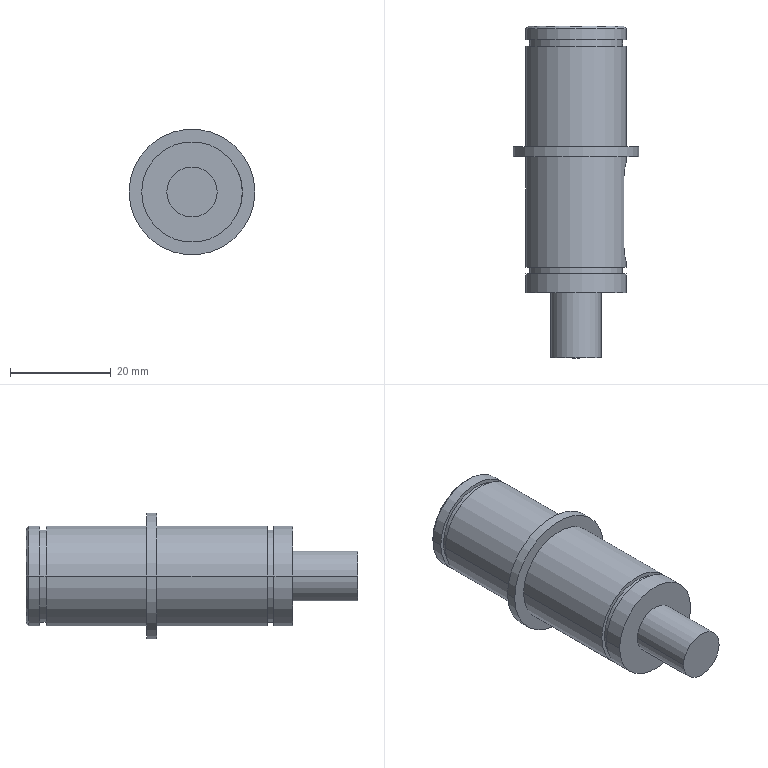Part | NX | features BREP 1 | 1 solid | 33 faces | box 25 x 66 x 25 mm | volume 17523 mm3 | cylinder 19 | plane 12 | cone 2 | commonest cylinder face diameters 20 x8 18.5 x4 6 x3 10 x2 25 x2
STEP:
#1=CARTESIAN_POINT('',(-9.5,66.,0.));
#2=VERTEX_POINT('',#1);
#3=CARTESIAN_POINT('',(9.5,66.,0.));
#4=VERTEX_POINT('',#3);
#5=CARTESIAN_POINT('',(0.,66.,0.));
#6=DIRECTION('',(0.,1.,0.));
#7=DIRECTION('',(-1.,0.,0.));
#8=AXIS2_PLACEMENT_3D('',#5,#6,#7);
#9=CIRCLE('',#8,9.5);
#10=EDGE_CURVE('',#2,#4,#9,.T.);
#11=ORIENTED_EDGE('',*,*,#10,.F.);
#12=CARTESIAN_POINT('',(-10.,65.5,0.));
#13=VERTEX_POINT('',#12);
#14=CARTESIAN_POINT('',(-10.,65.5,0.));
#15=DIRECTION('',(-0.7071,-0.7071,0.));
#16=VECTOR('',#15,1000.);
#17=LINE('',#14,#16);
#18=EDGE_CURVE('',#2,#13,#17,.T.);
#19=ORIENTED_EDGE('',*,*,#18,.T.);
#20=CARTESIAN_POINT('',(10.,65.5,0.));
#21=VERTEX_POINT('',#20);
#22=CARTESIAN_POINT('',(0.,65.5,0.));
#23=DIRECTION('',(0.,-1.,0.));
#24=DIRECTION('',(-1.,0.,0.));
#25=AXIS2_PLACEMENT_3D('',#22,#23,#24);
#26=CIRCLE('',#25,10.);
#27=EDGE_CURVE('',#21,#13,#26,.T.);
#28=ORIENTED_EDGE('',*,*,#27,.F.);
#29=CARTESIAN_POINT('',(10.,65.5,0.));
#30=DIRECTION('',(0.7071,-0.7071,0.));
#31=VECTOR('',#30,1000.);
#32=LINE('',#29,#31);
#33=EDGE_CURVE('',#4,#21,#32,.T.);
#34=ORIENTED_EDGE('',*,*,#33,.F.);
#35=EDGE_LOOP('',(#11,#19,#28,#34));
#36=FACE_BOUND('',#35,.T.);
#37=CARTESIAN_POINT('',(0.,65.5,0.));
#38=DIRECTION('',(0.,-1.,0.));
#39=DIRECTION('',(-1.,0.,0.));
#40=AXIS2_PLACEMENT_3D('',#37,#38,#39);
#41=CONICAL_SURFACE('',#40,10.,0.7854);
#42=ADVANCED_FACE('',(#36),#41,.T.);
#43=ORIENTED_EDGE('',*,*,#27,.T.);
#44=CARTESIAN_POINT('',(-10.,63.3,0.));
#45=VERTEX_POINT('',#44);
#46=CARTESIAN_POINT('',(-10.,0.,0.));
#47=DIRECTION('',(0.,-1.,0.));
#48=VECTOR('',#47,1000.);
#49=LINE('',#46,#48);
#50=EDGE_CURVE('',#13,#45,#49,.T.);
#51=ORIENTED_EDGE('',*,*,#50,.T.);
#52=CARTESIAN_POINT('',(10.,63.3,0.));
#53=VERTEX_POINT('',#52);
#54=CARTESIAN_POINT('',(0.,63.3,0.));
#55=DIRECTION('',(0.,-1.,0.));
#56=DIRECTION('',(1.,0.,0.));
#57=AXIS2_PLACEMENT_3D('',#54,#55,#56);
#58=CIRCLE('',#57,10.);
#59=EDGE_CURVE('',#53,#45,#58,.T.);
#60=ORIENTED_EDGE('',*,*,#59,.F.);
#61=CARTESIAN_POINT('',(10.,0.,0.));
#62=DIRECTION('',(0.,-1.,0.));
#63=VECTOR('',#62,1000.);
#64=LINE('',#61,#63);
#65=EDGE_CURVE('',#21,#53,#64,.T.);
#66=ORIENTED_EDGE('',*,*,#65,.F.);
#67=EDGE_LOOP('',(#43,#51,#60,#66));
#68=FACE_BOUND('',#67,.T.);
#69=CARTESIAN_POINT('',(0.,0.,0.));
#70=DIRECTION('',(0.,-1.,0.));
#71=DIRECTION('',(-1.,0.,0.));
#72=AXIS2_PLACEMENT_3D('',#69,#70,#71);
#73=CYLINDRICAL_SURFACE('',#72,10.);
#74=ADVANCED_FACE('',(#68),#73,.T.);
#75=CARTESIAN_POINT('',(9.25,62.,0.));
#76=VERTEX_POINT('',#75);
#77=CARTESIAN_POINT('',(-9.25,62.,0.));
#78=VERTEX_POINT('',#77);
#79=CARTESIAN_POINT('',(0.,62.,0.));
#80=DIRECTION('',(0.,-1.,0.));
#81=DIRECTION('',(1.,0.,0.));
#82=AXIS2_PLACEMENT_3D('',#79,#80,#81);
#83=CIRCLE('',#82,9.25);
#84=EDGE_CURVE('',#76,#78,#83,.T.);
#85=ORIENTED_EDGE('',*,*,#84,.F.);
#86=CARTESIAN_POINT('',(9.25,63.3,0.));
#87=VERTEX_POINT('',#86);
#88=CARTESIAN_POINT('',(9.25,62.,0.));
#89=DIRECTION('',(0.,1.,0.));
#90=VECTOR('',#89,1000.);
#91=LINE('',#88,#90);
#92=EDGE_CURVE('',#87,#76,#91,.F.);
#93=ORIENTED_EDGE('',*,*,#92,.F.);
#94=CARTESIAN_POINT('',(-9.25,63.3,0.));
#95=VERTEX_POINT('',#94);
#96=CARTESIAN_POINT('',(0.,63.3,0.));
#97=DIRECTION('',(0.,-1.,0.));
#98=DIRECTION('',(1.,0.,0.));
#99=AXIS2_PLACEMENT_3D('',#96,#97,#98);
#100=CIRCLE('',#99,9.25);
#101=EDGE_CURVE('',#87,#95,#100,.T.);
#102=ORIENTED_EDGE('',*,*,#101,.T.);
#103=CARTESIAN_POINT('',(-9.25,62.,0.));
#104=DIRECTION('',(0.,1.,0.));
#105=VECTOR('',#104,1000.);
#106=LINE('',#103,#105);
#107=EDGE_CURVE('',#95,#78,#106,.F.);
#108=ORIENTED_EDGE('',*,*,#107,.T.);
#109=EDGE_LOOP('',(#85,#93,#102,#108));
#110=FACE_BOUND('',#109,.T.);
#111=CARTESIAN_POINT('',(0.,62.,0.));
#112=DIRECTION('',(0.,1.,0.));
#113=DIRECTION('',(1.,0.,0.));
#114=AXIS2_PLACEMENT_3D('',#111,#112,#113);
#115=CYLINDRICAL_SURFACE('',#114,9.25);
#116=ADVANCED_FACE('',(#110),#115,.T.);
#117=CARTESIAN_POINT('',(10.,16.7,0.));
#118=VERTEX_POINT('',#117);
#119=CARTESIAN_POINT('',(-10.,16.7,0.));
#120=VERTEX_POINT('',#119);
#121=CARTESIAN_POINT('',(0.,16.7,0.));
#122=DIRECTION('',(0.,-1.,0.));
#123=DIRECTION('',(1.,0.,0.));
#124=AXIS2_PLACEMENT_3D('',#121,#122,#123);
#125=CIRCLE('',#124,10.);
#126=EDGE_CURVE('',#118,#120,#125,.T.);
#127=ORIENTED_EDGE('',*,*,#126,.T.);
#128=CARTESIAN_POINT('',(-10.,13.,0.));
#129=VERTEX_POINT('',#128);
#130=CARTESIAN_POINT('',(-10.,0.,0.));
#131=DIRECTION('',(0.,-1.,0.));
#132=VECTOR('',#131,1000.);
#133=LINE('',#130,#132);
#134=EDGE_CURVE('',#120,#129,#133,.T.);
#135=ORIENTED_EDGE('',*,*,#134,.T.);
#136=CARTESIAN_POINT('',(10.,13.,0.));
#137=VERTEX_POINT('',#136);
#138=CARTESIAN_POINT('',(0.,13.,0.));
#139=DIRECTION('',(0.,-1.,0.));
#140=DIRECTION('',(1.,0.,0.));
#141=AXIS2_PLACEMENT_3D('',#138,#139,#140);
#142=CIRCLE('',#141,10.);
#143=EDGE_CURVE('',#137,#129,#142,.T.);
#144=ORIENTED_EDGE('',*,*,#143,.F.);
#145=CARTESIAN_POINT('',(10.,0.,0.));
#146=DIRECTION('',(0.,-1.,0.));
#147=VECTOR('',#146,1000.);
#148=LINE('',#145,#147);
#149=EDGE_CURVE('',#118,#137,#148,.T.);
#150=ORIENTED_EDGE('',*,*,#149,.F.);
#151=EDGE_LOOP('',(#127,#135,#144,#150));
#152=FACE_BOUND('',#151,.T.);
#153=CARTESIAN_POINT('',(0.,0.,0.));
#154=DIRECTION('',(0.,-1.,0.));
#155=DIRECTION('',(-1.,0.,0.));
#156=AXIS2_PLACEMENT_3D('',#153,#154,#155);
#157=CYLINDRICAL_SURFACE('',#156,10.);
#158=ADVANCED_FACE('',(#152),#157,.T.);
#159=CARTESIAN_POINT('',(5.,13.,0.));
#160=VERTEX_POINT('',#159);
#161=CARTESIAN_POINT('',(-5.,13.,0.));
#162=VERTEX_POINT('',#161);
#163=CARTESIAN_POINT('',(0.,13.,0.));
#164=DIRECTION('',(0.,-1.,0.));
#165=DIRECTION('',(1.,0.,0.));
#166=AXIS2_PLACEMENT_3D('',#163,#164,#165);
#167=CIRCLE('',#166,5.);
#168=EDGE_CURVE('',#160,#162,#167,.T.);
#169=ORIENTED_EDGE('',*,*,#168,.T.);
#170=CARTESIAN_POINT('',(-5.,0.,0.));
#171=VERTEX_POINT('',#170);
#172=CARTESIAN_POINT('',(-5.,0.,0.));
#173=DIRECTION('',(0.,-1.,0.));
#174=VECTOR('',#173,1000.);
#175=LINE('',#172,#174);
#176=EDGE_CURVE('',#162,#171,#175,.T.);
#177=ORIENTED_EDGE('',*,*,#176,.T.);
#178=CARTESIAN_POINT('',(5.,0.,0.));
#179=VERTEX_POINT('',#178);
#180=CARTESIAN_POINT('',(0.,0.,0.));
#181=DIRECTION('',(0.,-1.,0.));
#182=DIRECTION('',(1.,0.,0.));
#183=AXIS2_PLACEMENT_3D('',#180,#181,#182);
#184=CIRCLE('',#183,5.);
#185=EDGE_CURVE('',#179,#171,#184,.T.);
#186=ORIENTED_EDGE('',*,*,#185,.F.);
#187=CARTESIAN_POINT('',(5.,0.,0.));
#188=DIRECTION('',(0.,-1.,0.));
#189=VECTOR('',#188,1000.);
#190=LINE('',#187,#189);
#191=EDGE_CURVE('',#160,#179,#190,.T.);
#192=ORIENTED_EDGE('',*,*,#191,.F.);
#193=EDGE_LOOP('',(#169,#177,#186,#192));
#194=FACE_BOUND('',#193,.T.);
#195=CARTESIAN_POINT('',(0.,0.,0.));
#196=DIRECTION('',(0.,-1.,0.));
#197=DIRECTION('',(-1.,0.,0.));
#198=AXIS2_PLACEMENT_3D('',#195,#196,#197);
#199=CYLINDRICAL_SURFACE('',#198,5.);
#200=ADVANCED_FACE('',(#194),#199,.T.);
#201=CARTESIAN_POINT('',(9.25,16.7,0.));
#202=VERTEX_POINT('',#201);
#203=CARTESIAN_POINT('',(-9.25,16.7,0.));
#204=VERTEX_POINT('',#203);
#205=CARTESIAN_POINT('',(0.,16.7,0.));
#206=DIRECTION('',(0.,-1.,0.));
#207=DIRECTION('',(1.,0.,0.));
#208=AXIS2_PLACEMENT_3D('',#205,#206,#207);
#209=CIRCLE('',#208,9.25);
#210=EDGE_CURVE('',#202,#204,#209,.T.);
#211=ORIENTED_EDGE('',*,*,#210,.F.);
#212=CARTESIAN_POINT('',(9.25,18.,0.));
#213=VERTEX_POINT('',#212);
#214=CARTESIAN_POINT('',(9.25,16.7,0.));
#215=DIRECTION('',(0.,1.,0.));
#216=VECTOR('',#215,1000.);
#217=LINE('',#214,#216);
#218=EDGE_CURVE('',#213,#202,#217,.F.);
#219=ORIENTED_EDGE('',*,*,#218,.F.);
#220=CARTESIAN_POINT('',(-9.25,18.,0.));
#221=VERTEX_POINT('',#220);
#222=CARTESIAN_POINT('',(0.,18.,0.));
#223=DIRECTION('',(0.,-1.,0.));
#224=DIRECTION('',(1.,0.,0.));
#225=AXIS2_PLACEMENT_3D('',#222,#223,#224);
#226=CIRCLE('',#225,9.25);
#227=EDGE_CURVE('',#213,#221,#226,.T.);
#228=ORIENTED_EDGE('',*,*,#227,.T.);
#229=CARTESIAN_POINT('',(-9.25,16.7,0.));
#230=DIRECTION('',(0.,1.,0.));
#231=VECTOR('',#230,1000.);
#232=LINE('',#229,#231);
#233=EDGE_CURVE('',#221,#204,#232,.F.);
#234=ORIENTED_EDGE('',*,*,#233,.T.);
#235=EDGE_LOOP('',(#211,#219,#228,#234));
#236=FACE_BOUND('',#235,.T.);
#237=CARTESIAN_POINT('',(0.,16.7,0.));
#238=DIRECTION('',(0.,1.,0.));
#239=DIRECTION('',(1.,0.,0.));
#240=AXIS2_PLACEMENT_3D('',#237,#238,#239);
#241=CYLINDRICAL_SURFACE('',#240,9.25);
#242=ADVANCED_FACE('',(#236),#241,.T.);
#243=CARTESIAN_POINT('',(6.5,39.,0.));
#244=VERTEX_POINT('',#243);
#245=CARTESIAN_POINT('',(6.5,36.,3.));
#246=VERTEX_POINT('',#245);
#247=CARTESIAN_POINT('',(6.5,36.,0.));
#248=DIRECTION('',(1.,0.,0.));
#249=DIRECTION('',(0.,1.,0.));
#250=AXIS2_PLACEMENT_3D('',#247,#248,#249);
#251=CIRCLE('',#250,3.);
#252=EDGE_CURVE('',#244,#246,#251,.T.);
#253=ORIENTED_EDGE('',*,*,#252,.F.);
#254=CARTESIAN_POINT('',(10.,39.,0.));
#255=VERTEX_POINT('',#254);
#256=CARTESIAN_POINT('',(6.5,39.,0.));
#257=DIRECTION('',(1.,0.,0.));
#258=VECTOR('',#257,1000.);
#259=LINE('',#256,#258);
#260=EDGE_CURVE('',#244,#255,#259,.T.);
#261=ORIENTED_EDGE('',*,*,#260,.T.);
#262=CARTESIAN_POINT('',(9.539,36.,3.));
#263=VERTEX_POINT('',#262);
#264=CARTESIAN_POINT('',(10.,39.,0.));
#265=CARTESIAN_POINT('',(10.,39.,0.7973));
#266=CARTESIAN_POINT('',(9.775,38.345,2.343));
#267=CARTESIAN_POINT('',(9.539,36.797,3.));
#268=CARTESIAN_POINT('',(9.539,36.,3.));
#269=B_SPLINE_CURVE_WITH_KNOTS('',3,(#264,#265,#266,#267,#268),.UNSPECIFIED.,.F.,.F.,(4,1,4),(0.,0.002357,0.004714),.UNSPECIFIED.);
#270=EDGE_CURVE('',#255,#263,#269,.T.);
#271=ORIENTED_EDGE('',*,*,#270,.T.);
#272=CARTESIAN_POINT('',(6.5,36.,3.));
#273=DIRECTION('',(1.,0.,0.));
#274=VECTOR('',#273,1000.);
#275=LINE('',#272,#274);
#276=EDGE_CURVE('',#246,#263,#275,.T.);
#277=ORIENTED_EDGE('',*,*,#276,.F.);
#278=EDGE_LOOP('',(#253,#261,#271,#277));
#279=FACE_BOUND('',#278,.T.);
#280=CARTESIAN_POINT('',(6.5,36.,0.));
#281=DIRECTION('',(1.,0.,0.));
#282=DIRECTION('',(0.,-1.,0.));
#283=AXIS2_PLACEMENT_3D('',#280,#281,#282);
#284=CYLINDRICAL_SURFACE('',#283,3.);
#285=ADVANCED_FACE('',(#279),#284,.F.);
#286=CARTESIAN_POINT('',(12.5,42.,0.));
#287=VERTEX_POINT('',#286);
#288=CARTESIAN_POINT('',(-12.5,42.,0.));
#289=VERTEX_POINT('',#288);
#290=CARTESIAN_POINT('',(0.,42.,0.));
#291=DIRECTION('',(0.,-1.,0.));
#292=DIRECTION('',(1.,0.,0.));
#293=AXIS2_PLACEMENT_3D('',#290,#291,#292);
#294=CIRCLE('',#293,12.5);
#295=EDGE_CURVE('',#287,#289,#294,.T.);
#296=ORIENTED_EDGE('',*,*,#295,.T.);
#297=CARTESIAN_POINT('',(-12.5,40.,0.));
#298=VERTEX_POINT('',#297);
#299=CARTESIAN_POINT('',(-12.5,0.,0.));
#300=DIRECTION('',(0.,-1.,0.));
#301=VECTOR('',#300,1000.);
#302=LINE('',#299,#301);
#303=EDGE_CURVE('',#289,#298,#302,.T.);
#304=ORIENTED_EDGE('',*,*,#303,.T.);
#305=CARTESIAN_POINT('',(12.5,40.,0.));
#306=VERTEX_POINT('',#305);
#307=CARTESIAN_POINT('',(0.,40.,0.));
#308=DIRECTION('',(0.,-1.,0.));
#309=DIRECTION('',(1.,0.,0.));
#310=AXIS2_PLACEMENT_3D('',#307,#308,#309);
#311=CIRCLE('',#310,12.5);
#312=EDGE_CURVE('',#306,#298,#311,.T.);
#313=ORIENTED_EDGE('',*,*,#312,.F.);
#314=CARTESIAN_POINT('',(12.5,0.,0.));
#315=DIRECTION('',(0.,-1.,0.));
#316=VECTOR('',#315,1000.);
#317=LINE('',#314,#316);
#318=EDGE_CURVE('',#287,#306,#317,.T.);
#319=ORIENTED_EDGE('',*,*,#318,.F.);
#320=EDGE_LOOP('',(#296,#304,#313,#319));
#321=FACE_BOUND('',#320,.T.);
#322=CARTESIAN_POINT('',(0.,0.,0.));
#323=DIRECTION('',(0.,-1.,0.));
#324=DIRECTION('',(-1.,0.,0.));
#325=AXIS2_PLACEMENT_3D('',#322,#323,#324);
#326=CYLINDRICAL_SURFACE('',#325,12.5);
#327=ADVANCED_FACE('',(#321),#326,.T.);
#328=CARTESIAN_POINT('',(10.,62.,0.));
#329=VERTEX_POINT('',#328);
#330=CARTESIAN_POINT('',(-10.,62.,0.));
#331=VERTEX_POINT('',#330);
#332=CARTESIAN_POINT('',(0.,62.,0.));
#333=DIRECTION('',(0.,-1.,0.));
#334=DIRECTION('',(1.,0.,0.));
#335=AXIS2_PLACEMENT_3D('',#332,#333,#334);
#336=CIRCLE('',#335,10.);
#337=EDGE_CURVE('',#329,#331,#336,.T.);
#338=ORIENTED_EDGE('',*,*,#337,.T.);
#339=CARTESIAN_POINT('',(-10.,42.,0.));
#340=VERTEX_POINT('',#339);
#341=CARTESIAN_POINT('',(-10.,0.,0.));
#342=DIRECTION('',(0.,-1.,0.));
#343=VECTOR('',#342,1000.);
#344=LINE('',#341,#343);
#345=EDGE_CURVE('',#331,#340,#344,.T.);
#346=ORIENTED_EDGE('',*,*,#345,.T.);
#347=CARTESIAN_POINT('',(10.,42.,0.));
#348=VERTEX_POINT('',#347);
#349=CARTESIAN_POINT('',(0.,42.,0.));
#350=DIRECTION('',(0.,-1.,0.));
#351=DIRECTION('',(1.,0.,0.));
#352=AXIS2_PLACEMENT_3D('',#349,#350,#351);
#353=CIRCLE('',#352,10.);
#354=EDGE_CURVE('',#348,#340,#353,.T.);
#355=ORIENTED_EDGE('',*,*,#354,.F.);
#356=CARTESIAN_POINT('',(10.,0.,0.));
#357=DIRECTION('',(0.,-1.,0.));
#358=VECTOR('',#357,1000.);
#359=LINE('',#356,#358);
#360=EDGE_CURVE('',#329,#348,#359,.T.);
#361=ORIENTED_EDGE('',*,*,#360,.F.);
#362=EDGE_LOOP('',(#338,#346,#355,#361));
#363=FACE_BOUND('',#362,.T.);
#364=CARTESIAN_POINT('',(0.,0.,0.));
#365=DIRECTION('',(0.,-1.,0.));
#366=DIRECTION('',(-1.,0.,0.));
#367=AXIS2_PLACEMENT_3D('',#364,#365,#366);
#368=CYLINDRICAL_SURFACE('',#367,10.);
#369=ADVANCED_FACE('',(#363),#368,.T.);
#370=CARTESIAN_POINT('',(10.,40.,0.));
#371=VERTEX_POINT('',#370);
#372=CARTESIAN_POINT('',(-10.,40.,0.));
#373=VERTEX_POINT('',#372);
#374=CARTESIAN_POINT('',(0.,40.,0.));
#375=DIRECTION('',(0.,-1.,0.));
#376=DIRECTION('',(1.,0.,0.));
#377=AXIS2_PLACEMENT_3D('',#374,#375,#376);
#378=CIRCLE('',#377,10.);
#379=EDGE_CURVE('',#371,#373,#378,.T.);
#380=ORIENTED_EDGE('',*,*,#379,.T.);
#381=CARTESIAN_POINT('',(-10.,18.,0.));
#382=VERTEX_POINT('',#381);
#383=CARTESIAN_POINT('',(-10.,0.,0.));
#384=DIRECTION('',(0.,-1.,0.));
#385=VECTOR('',#384,1000.);
#386=LINE('',#383,#385);
#387=EDGE_CURVE('',#373,#382,#386,.T.);
#388=ORIENTED_EDGE('',*,*,#387,.T.);
#389=CARTESIAN_POINT('',(10.,18.,0.));
#390=VERTEX_POINT('',#389);
#391=CARTESIAN_POINT('',(0.,18.,0.));
#392=DIRECTION('',(0.,-1.,0.));
#393=DIRECTION('',(1.,0.,0.));
#394=AXIS2_PLACEMENT_3D('',#391,#392,#393);
#395=CIRCLE('',#394,10.);
#396=EDGE_CURVE('',#390,#382,#395,.T.);
#397=ORIENTED_EDGE('',*,*,#396,.F.);
#398=CARTESIAN_POINT('',(10.,19.,0.));
#399=VERTEX_POINT('',#398);
#400=CARTESIAN_POINT('',(10.,0.,0.));
#401=DIRECTION('',(0.,-1.,0.));
#402=VECTOR('',#401,1000.);
#403=LINE('',#400,#402);
#404=EDGE_CURVE('',#399,#390,#403,.T.);
#405=ORIENTED_EDGE('',*,*,#404,.F.);
#406=CARTESIAN_POINT('',(9.539,22.,3.));
#407=VERTEX_POINT('',#406);
#408=CARTESIAN_POINT('',(9.539,22.,3.));
#409=CARTESIAN_POINT('',(9.539,21.203,3.));
#410=CARTESIAN_POINT('',(9.775,19.657,2.345));
#411=CARTESIAN_POINT('',(10.,19.,0.7973));
#412=CARTESIAN_POINT('',(10.,19.,0.));
#413=B_SPLINE_CURVE_WITH_KNOTS('',3,(#408,#409,#410,#411,#412),.UNSPECIFIED.,.F.,.F.,(4,1,4),(0.,0.002357,0.004714),.UNSPECIFIED.);
#414=EDGE_CURVE('',#407,#399,#413,.T.);
#415=ORIENTED_EDGE('',*,*,#414,.F.);
#416=CARTESIAN_POINT('',(9.539,0.,3.));
#417=DIRECTION('',(0.,-1.,0.));
#418=VECTOR('',#417,1000.);
#419=LINE('',#416,#418);
#420=EDGE_CURVE('',#263,#407,#419,.T.);
#421=ORIENTED_EDGE('',*,*,#420,.F.);
#422=ORIENTED_EDGE('',*,*,#270,.F.);
#423=CARTESIAN_POINT('',(10.,0.,0.));
#424=DIRECTION('',(0.,-1.,0.));
#425=VECTOR('',#424,1000.);
#426=LINE('',#423,#425);
#427=EDGE_CURVE('',#371,#255,#426,.T.);
#428=ORIENTED_EDGE('',*,*,#427,.F.);
#429=EDGE_LOOP('',(#380,#388,#397,#405,#415,#421,#422,#428));
#430=FACE_BOUND('',#429,.T.);
#431=CARTESIAN_POINT('',(0.,0.,0.));
#432=DIRECTION('',(0.,-1.,0.));
#433=DIRECTION('',(-1.,0.,0.));
#434=AXIS2_PLACEMENT_3D('',#431,#432,#433);
#435=CYLINDRICAL_SURFACE('',#434,10.);
#436=ADVANCED_FACE('',(#430),#435,.T.);
#437=ORIENTED_EDGE('',*,*,#387,.F.);
#438=CARTESIAN_POINT('',(0.,40.,0.));
#439=DIRECTION('',(0.,-1.,0.));
#440=DIRECTION('',(1.,0.,0.));
#441=AXIS2_PLACEMENT_3D('',#438,#439,#440);
#442=CIRCLE('',#441,10.);
#443=EDGE_CURVE('',#373,#371,#442,.T.);
#444=ORIENTED_EDGE('',*,*,#443,.T.);
#445=ORIENTED_EDGE('',*,*,#427,.T.);
#446=CARTESIAN_POINT('',(9.539,36.,-3.));
#447=VERTEX_POINT('',#446);
#448=CARTESIAN_POINT('',(9.539,36.,-3.));
#449=CARTESIAN_POINT('',(9.539,36.797,-3.));
#450=CARTESIAN_POINT('',(9.775,38.343,-2.345));
#451=CARTESIAN_POINT('',(10.,39.,-0.7973));
#452=CARTESIAN_POINT('',(10.,39.,0.));
#453=B_SPLINE_CURVE_WITH_KNOTS('',3,(#448,#449,#450,#451,#452),.UNSPECIFIED.,.F.,.F.,(4,1,4),(0.,0.002357,0.004714),.UNSPECIFIED.);
#454=EDGE_CURVE('',#447,#255,#453,.T.);
#455=ORIENTED_EDGE('',*,*,#454,.F.);
#456=CARTESIAN_POINT('',(9.539,22.,-3.));
#457=VERTEX_POINT('',#456);
#458=CARTESIAN_POINT('',(9.539,0.,-3.));
#459=DIRECTION('',(0.,1.,0.));
#460=VECTOR('',#459,1000.);
#461=LINE('',#458,#460);
#462=EDGE_CURVE('',#457,#447,#461,.T.);
#463=ORIENTED_EDGE('',*,*,#462,.F.);
#464=CARTESIAN_POINT('',(10.,19.,0.));
#465=CARTESIAN_POINT('',(10.,19.,-0.7973));
#466=CARTESIAN_POINT('',(9.775,19.655,-2.343));
#467=CARTESIAN_POINT('',(9.539,21.203,-3.));
#468=CARTESIAN_POINT('',(9.539,22.,-3.));
#469=B_SPLINE_CURVE_WITH_KNOTS('',3,(#464,#465,#466,#467,#468),.UNSPECIFIED.,.F.,.F.,(4,1,4),(0.,0.002357,0.004714),.UNSPECIFIED.);
#470=EDGE_CURVE('',#399,#457,#469,.T.);
#471=ORIENTED_EDGE('',*,*,#470,.F.);
#472=ORIENTED_EDGE('',*,*,#404,.T.);
#473=CARTESIAN_POINT('',(0.,18.,0.));
#474=DIRECTION('',(0.,-1.,0.));
#475=DIRECTION('',(1.,0.,0.));
#476=AXIS2_PLACEMENT_3D('',#473,#474,#475);
#477=CIRCLE('',#476,10.);
#478=EDGE_CURVE('',#382,#390,#477,.T.);
#479=ORIENTED_EDGE('',*,*,#478,.F.);
#480=EDGE_LOOP('',(#437,#444,#445,#455,#463,#471,#472,#479));
#481=FACE_BOUND('',#480,.T.);
#482=CARTESIAN_POINT('',(0.,0.,0.));
#483=DIRECTION('',(0.,-1.,0.));
#484=DIRECTION('',(-1.,0.,0.));
#485=AXIS2_PLACEMENT_3D('',#482,#483,#484);
#486=CYLINDRICAL_SURFACE('',#485,10.);
#487=ADVANCED_FACE('',(#481),#486,.T.);
#488=ORIENTED_EDGE('',*,*,#345,.F.);
#489=CARTESIAN_POINT('',(0.,62.,0.));
#490=DIRECTION('',(0.,-1.,0.));
#491=DIRECTION('',(1.,0.,0.));
#492=AXIS2_PLACEMENT_3D('',#489,#490,#491);
#493=CIRCLE('',#492,10.);
#494=EDGE_CURVE('',#331,#329,#493,.T.);
#495=ORIENTED_EDGE('',*,*,#494,.T.);
#496=ORIENTED_EDGE('',*,*,#360,.T.);
#497=CARTESIAN_POINT('',(0.,42.,0.));
#498=DIRECTION('',(0.,-1.,0.));
#499=DIRECTION('',(1.,0.,0.));
#500=AXIS2_PLACEMENT_3D('',#497,#498,#499);
#501=CIRCLE('',#500,10.);
#502=EDGE_CURVE('',#340,#348,#501,.T.);
#503=ORIENTED_EDGE('',*,*,#502,.F.);
#504=EDGE_LOOP('',(#488,#495,#496,#503));
#505=FACE_BOUND('',#504,.T.);
#506=CARTESIAN_POINT('',(0.,0.,0.));
#507=DIRECTION('',(0.,-1.,0.));
#508=DIRECTION('',(-1.,0.,0.));
#509=AXIS2_PLACEMENT_3D('',#506,#507,#508);
#510=CYLINDRICAL_SURFACE('',#509,10.);
#511=ADVANCED_FACE('',(#505),#510,.T.);
#512=ORIENTED_EDGE('',*,*,#354,.T.);
#513=ORIENTED_EDGE('',*,*,#502,.T.);
#514=EDGE_LOOP('',(#512,#513));
#515=FACE_BOUND('',#514,.T.);
#516=ORIENTED_EDGE('',*,*,#295,.F.);
#517=CARTESIAN_POINT('',(0.,42.,0.));
#518=DIRECTION('',(0.,-1.,0.));
#519=DIRECTION('',(1.,0.,0.));
#520=AXIS2_PLACEMENT_3D('',#517,#518,#519);
#521=CIRCLE('',#520,12.5);
#522=EDGE_CURVE('',#289,#287,#521,.T.);
#523=ORIENTED_EDGE('',*,*,#522,.F.);
#524=EDGE_LOOP('',(#516,#523));
#525=FACE_BOUND('',#524,.T.);
#526=CARTESIAN_POINT('',(10.,42.,0.));
#527=DIRECTION('',(0.,1.,0.));
#528=DIRECTION('',(1.,0.,0.));
#529=AXIS2_PLACEMENT_3D('',#526,#527,#528);
#530=PLANE('',#529);
#531=ADVANCED_FACE('',(#515,#525),#530,.T.);
#532=ORIENTED_EDGE('',*,*,#303,.F.);
#533=ORIENTED_EDGE('',*,*,#522,.T.);
#534=ORIENTED_EDGE('',*,*,#318,.T.);
#535=CARTESIAN_POINT('',(0.,40.,0.));
#536=DIRECTION('',(0.,-1.,0.));
#537=DIRECTION('',(1.,0.,0.));
#538=AXIS2_PLACEMENT_3D('',#535,#536,#537);
#539=CIRCLE('',#538,12.5);
#540=EDGE_CURVE('',#298,#306,#539,.T.);
#541=ORIENTED_EDGE('',*,*,#540,.F.);
#542=EDGE_LOOP('',(#532,#533,#534,#541));
#543=FACE_BOUND('',#542,.T.);
#544=CARTESIAN_POINT('',(0.,0.,0.));
#545=DIRECTION('',(0.,-1.,0.));
#546=DIRECTION('',(-1.,0.,0.));
#547=AXIS2_PLACEMENT_3D('',#544,#545,#546);
#548=CYLINDRICAL_SURFACE('',#547,12.5);
#549=ADVANCED_FACE('',(#543),#548,.T.);
#550=ORIENTED_EDGE('',*,*,#312,.T.);
#551=ORIENTED_EDGE('',*,*,#540,.T.);
#552=EDGE_LOOP('',(#550,#551));
#553=FACE_BOUND('',#552,.T.);
#554=ORIENTED_EDGE('',*,*,#379,.F.);
#555=ORIENTED_EDGE('',*,*,#443,.F.);
#556=EDGE_LOOP('',(#554,#555));
#557=FACE_BOUND('',#556,.T.);
#558=CARTESIAN_POINT('',(12.5,40.,0.));
#559=DIRECTION('',(0.,-1.,0.));
#560=DIRECTION('',(-1.,0.,0.));
#561=AXIS2_PLACEMENT_3D('',#558,#559,#560);
#562=PLANE('',#561);
#563=ADVANCED_FACE('',(#553,#557),#562,.T.);
#564=ORIENTED_EDGE('',*,*,#260,.F.);
#565=CARTESIAN_POINT('',(6.5,36.,-3.));
#566=VERTEX_POINT('',#565);
#567=CARTESIAN_POINT('',(6.5,36.,0.));
#568=DIRECTION('',(1.,0.,0.));
#569=DIRECTION('',(0.,1.,0.));
#570=AXIS2_PLACEMENT_3D('',#567,#568,#569);
#571=CIRCLE('',#570,3.);
#572=EDGE_CURVE('',#566,#244,#571,.T.);
#573=ORIENTED_EDGE('',*,*,#572,.F.);
#574=CARTESIAN_POINT('',(6.5,36.,-3.));
#575=DIRECTION('',(1.,0.,0.));
#576=VECTOR('',#575,1000.);
#577=LINE('',#574,#576);
#578=EDGE_CURVE('',#566,#447,#577,.T.);
#579=ORIENTED_EDGE('',*,*,#578,.T.);
#580=ORIENTED_EDGE('',*,*,#454,.T.);
#581=EDGE_LOOP('',(#564,#573,#579,#580));
#582=FACE_BOUND('',#581,.T.);
#583=CARTESIAN_POINT('',(6.5,36.,0.));
#584=DIRECTION('',(1.,0.,0.));
#585=DIRECTION('',(0.,-1.,0.));
#586=AXIS2_PLACEMENT_3D('',#583,#584,#585);
#587=CYLINDRICAL_SURFACE('',#586,3.);
#588=ADVANCED_FACE('',(#582),#587,.F.);
#589=ORIENTED_EDGE('',*,*,#462,.T.);
#590=ORIENTED_EDGE('',*,*,#578,.F.);
#591=CARTESIAN_POINT('',(6.5,22.,-3.));
#592=VERTEX_POINT('',#591);
#593=CARTESIAN_POINT('',(6.5,36.,-3.));
#594=DIRECTION('',(0.,1.,0.));
#595=VECTOR('',#594,1000.);
#596=LINE('',#593,#595);
#597=EDGE_CURVE('',#592,#566,#596,.T.);
#598=ORIENTED_EDGE('',*,*,#597,.F.);
#599=CARTESIAN_POINT('',(6.5,22.,-3.));
#600=DIRECTION('',(1.,0.,0.));
#601=VECTOR('',#600,1000.);
#602=LINE('',#599,#601);
#603=EDGE_CURVE('',#592,#457,#602,.T.);
#604=ORIENTED_EDGE('',*,*,#603,.T.);
#605=EDGE_LOOP('',(#589,#590,#598,#604));
#606=FACE_BOUND('',#605,.T.);
#607=CARTESIAN_POINT('',(6.5,36.,-3.));
#608=DIRECTION('',(0.,0.,-1.));
#609=DIRECTION('',(0.,-1.,0.));
#610=AXIS2_PLACEMENT_3D('',#607,#608,#609);
#611=PLANE('',#610);
#612=ADVANCED_FACE('',(#606),#611,.F.);
#613=CARTESIAN_POINT('',(6.5,22.,3.));
#614=VERTEX_POINT('',#613);
#615=CARTESIAN_POINT('',(6.5,22.,3.));
#616=DIRECTION('',(1.,0.,0.));
#617=VECTOR('',#616,1000.);
#618=LINE('',#615,#617);
#619=EDGE_CURVE('',#614,#407,#618,.T.);
#620=ORIENTED_EDGE('',*,*,#619,.T.);
#621=ORIENTED_EDGE('',*,*,#414,.T.);
#622=ORIENTED_EDGE('',*,*,#470,.T.);
#623=ORIENTED_EDGE('',*,*,#603,.F.);
#624=CARTESIAN_POINT('',(6.5,22.,0.));
#625=DIRECTION('',(1.,0.,0.));
#626=DIRECTION('',(0.,1.,0.));
#627=AXIS2_PLACEMENT_3D('',#624,#625,#626);
#628=CIRCLE('',#627,3.);
#629=EDGE_CURVE('',#614,#592,#628,.T.);
#630=ORIENTED_EDGE('',*,*,#629,.F.);
#631=EDGE_LOOP('',(#620,#621,#622,#623,#630));
#632=FACE_BOUND('',#631,.T.);
#633=CARTESIAN_POINT('',(6.5,22.,0.));
#634=DIRECTION('',(1.,0.,0.));
#635=DIRECTION('',(0.,-1.,0.));
#636=AXIS2_PLACEMENT_3D('',#633,#634,#635);
#637=CYLINDRICAL_SURFACE('',#636,3.);
#638=ADVANCED_FACE('',(#632),#637,.F.);
#639=ORIENTED_EDGE('',*,*,#420,.T.);
#640=ORIENTED_EDGE('',*,*,#619,.F.);
#641=CARTESIAN_POINT('',(6.5,36.,3.));
#642=DIRECTION('',(0.,-1.,0.));
#643=VECTOR('',#642,1000.);
#644=LINE('',#641,#643);
#645=EDGE_CURVE('',#246,#614,#644,.T.);
#646=ORIENTED_EDGE('',*,*,#645,.F.);
#647=ORIENTED_EDGE('',*,*,#276,.T.);
#648=EDGE_LOOP('',(#639,#640,#646,#647));
#649=FACE_BOUND('',#648,.T.);
#650=CARTESIAN_POINT('',(6.5,36.,3.));
#651=DIRECTION('',(0.,0.,1.));
#652=DIRECTION('',(0.,1.,0.));
#653=AXIS2_PLACEMENT_3D('',#650,#651,#652);
#654=PLANE('',#653);
#655=ADVANCED_FACE('',(#649),#654,.F.);
#656=ORIENTED_EDGE('',*,*,#572,.T.);
#657=ORIENTED_EDGE('',*,*,#252,.T.);
#658=ORIENTED_EDGE('',*,*,#645,.T.);
#659=ORIENTED_EDGE('',*,*,#629,.T.);
#660=ORIENTED_EDGE('',*,*,#597,.T.);
#661=EDGE_LOOP('',(#656,#657,#658,#659,#660));
#662=FACE_BOUND('',#661,.T.);
#663=CARTESIAN_POINT('',(6.5,36.,0.));
#664=DIRECTION('',(1.,0.,0.));
#665=DIRECTION('',(0.,-1.,0.));
#666=AXIS2_PLACEMENT_3D('',#663,#664,#665);
#667=PLANE('',#666);
#668=ADVANCED_FACE('',(#662),#667,.T.);
#669=ORIENTED_EDGE('',*,*,#126,.F.);
#670=CARTESIAN_POINT('',(0.,16.7,0.));
#671=DIRECTION('',(0.,-1.,0.));
#672=DIRECTION('',(1.,0.,0.));
#673=AXIS2_PLACEMENT_3D('',#670,#671,#672);
#674=CIRCLE('',#673,10.);
#675=EDGE_CURVE('',#120,#118,#674,.T.);
#676=ORIENTED_EDGE('',*,*,#675,.F.);
#677=EDGE_LOOP('',(#669,#676));
#678=FACE_BOUND('',#677,.T.);
#679=CARTESIAN_POINT('',(0.,16.7,0.));
#680=DIRECTION('',(0.,-1.,0.));
#681=DIRECTION('',(1.,0.,0.));
#682=AXIS2_PLACEMENT_3D('',#679,#680,#681);
#683=CIRCLE('',#682,9.25);
#684=EDGE_CURVE('',#204,#202,#683,.T.);
#685=ORIENTED_EDGE('',*,*,#684,.T.);
#686=ORIENTED_EDGE('',*,*,#210,.T.);
#687=EDGE_LOOP('',(#685,#686));
#688=FACE_BOUND('',#687,.T.);
#689=CARTESIAN_POINT('',(0.,16.7,0.));
#690=DIRECTION('',(0.,-1.,0.));
#691=DIRECTION('',(-1.,0.,0.));
#692=AXIS2_PLACEMENT_3D('',#689,#690,#691);
#693=PLANE('',#692);
#694=ADVANCED_FACE('',(#678,#688),#693,.F.);
#695=ORIENTED_EDGE('',*,*,#396,.T.);
#696=ORIENTED_EDGE('',*,*,#478,.T.);
#697=EDGE_LOOP('',(#695,#696));
#698=FACE_BOUND('',#697,.T.);
#699=CARTESIAN_POINT('',(0.,18.,0.));
#700=DIRECTION('',(0.,-1.,0.));
#701=DIRECTION('',(1.,0.,0.));
#702=AXIS2_PLACEMENT_3D('',#699,#700,#701);
#703=CIRCLE('',#702,9.25);
#704=EDGE_CURVE('',#221,#213,#703,.T.);
#705=ORIENTED_EDGE('',*,*,#704,.F.);
#706=ORIENTED_EDGE('',*,*,#227,.F.);
#707=EDGE_LOOP('',(#705,#706));
#708=FACE_BOUND('',#707,.T.);
#709=CARTESIAN_POINT('',(0.,18.,0.));
#710=DIRECTION('',(0.,-1.,0.));
#711=DIRECTION('',(-1.,0.,0.));
#712=AXIS2_PLACEMENT_3D('',#709,#710,#711);
#713=PLANE('',#712);
#714=ADVANCED_FACE('',(#698,#708),#713,.T.);
#715=ORIENTED_EDGE('',*,*,#218,.T.);
#716=ORIENTED_EDGE('',*,*,#684,.F.);
#717=ORIENTED_EDGE('',*,*,#233,.F.);
#718=ORIENTED_EDGE('',*,*,#704,.T.);
#719=EDGE_LOOP('',(#715,#716,#717,#718));
#720=FACE_BOUND('',#719,.T.);
#721=CARTESIAN_POINT('',(0.,16.7,0.));
#722=DIRECTION('',(0.,1.,0.));
#723=DIRECTION('',(1.,0.,0.));
#724=AXIS2_PLACEMENT_3D('',#721,#722,#723);
#725=CYLINDRICAL_SURFACE('',#724,9.25);
#726=ADVANCED_FACE('',(#720),#725,.T.);
#727=ORIENTED_EDGE('',*,*,#185,.T.);
#728=CARTESIAN_POINT('',(0.,0.,0.));
#729=DIRECTION('',(0.,-1.,0.));
#730=DIRECTION('',(1.,0.,0.));
#731=AXIS2_PLACEMENT_3D('',#728,#729,#730);
#732=CIRCLE('',#731,5.);
#733=EDGE_CURVE('',#171,#179,#732,.T.);
#734=ORIENTED_EDGE('',*,*,#733,.T.);
#735=EDGE_LOOP('',(#727,#734));
#736=FACE_BOUND('',#735,.T.);
#737=CARTESIAN_POINT('',(5.,0.,0.));
#738=DIRECTION('',(0.,-1.,0.));
#739=DIRECTION('',(-1.,0.,0.));
#740=AXIS2_PLACEMENT_3D('',#737,#738,#739);
#741=PLANE('',#740);
#742=ADVANCED_FACE('',(#736),#741,.T.);
#743=ORIENTED_EDGE('',*,*,#176,.F.);
#744=CARTESIAN_POINT('',(0.,13.,0.));
#745=DIRECTION('',(0.,-1.,0.));
#746=DIRECTION('',(1.,0.,0.));
#747=AXIS2_PLACEMENT_3D('',#744,#745,#746);
#748=CIRCLE('',#747,5.);
#749=EDGE_CURVE('',#162,#160,#748,.T.);
#750=ORIENTED_EDGE('',*,*,#749,.T.);
#751=ORIENTED_EDGE('',*,*,#191,.T.);
#752=ORIENTED_EDGE('',*,*,#733,.F.);
#753=EDGE_LOOP('',(#743,#750,#751,#752));
#754=FACE_BOUND('',#753,.T.);
#755=CARTESIAN_POINT('',(0.,0.,0.));
#756=DIRECTION('',(0.,-1.,0.));
#757=DIRECTION('',(-1.,0.,0.));
#758=AXIS2_PLACEMENT_3D('',#755,#756,#757);
#759=CYLINDRICAL_SURFACE('',#758,5.);
#760=ADVANCED_FACE('',(#754),#759,.T.);
#761=ORIENTED_EDGE('',*,*,#143,.T.);
#762=CARTESIAN_POINT('',(0.,13.,0.));
#763=DIRECTION('',(0.,-1.,0.));
#764=DIRECTION('',(1.,0.,0.));
#765=AXIS2_PLACEMENT_3D('',#762,#763,#764);
#766=CIRCLE('',#765,10.);
#767=EDGE_CURVE('',#129,#137,#766,.T.);
#768=ORIENTED_EDGE('',*,*,#767,.T.);
#769=EDGE_LOOP('',(#761,#768));
#770=FACE_BOUND('',#769,.T.);
#771=ORIENTED_EDGE('',*,*,#168,.F.);
#772=ORIENTED_EDGE('',*,*,#749,.F.);
#773=EDGE_LOOP('',(#771,#772));
#774=FACE_BOUND('',#773,.T.);
#775=CARTESIAN_POINT('',(10.,13.,0.));
#776=DIRECTION('',(0.,-1.,0.));
#777=DIRECTION('',(-1.,0.,0.));
#778=AXIS2_PLACEMENT_3D('',#775,#776,#777);
#779=PLANE('',#778);
#780=ADVANCED_FACE('',(#770,#774),#779,.T.);
#781=ORIENTED_EDGE('',*,*,#134,.F.);
#782=ORIENTED_EDGE('',*,*,#675,.T.);
#783=ORIENTED_EDGE('',*,*,#149,.T.);
#784=ORIENTED_EDGE('',*,*,#767,.F.);
#785=EDGE_LOOP('',(#781,#782,#783,#784));
#786=FACE_BOUND('',#785,.T.);
#787=CARTESIAN_POINT('',(0.,0.,0.));
#788=DIRECTION('',(0.,-1.,0.));
#789=DIRECTION('',(-1.,0.,0.));
#790=AXIS2_PLACEMENT_3D('',#787,#788,#789);
#791=CYLINDRICAL_SURFACE('',#790,10.);
#792=ADVANCED_FACE('',(#786),#791,.T.);
#793=ORIENTED_EDGE('',*,*,#337,.F.);
#794=ORIENTED_EDGE('',*,*,#494,.F.);
#795=EDGE_LOOP('',(#793,#794));
#796=FACE_BOUND('',#795,.T.);
#797=CARTESIAN_POINT('',(0.,62.,0.));
#798=DIRECTION('',(0.,-1.,0.));
#799=DIRECTION('',(1.,0.,0.));
#800=AXIS2_PLACEMENT_3D('',#797,#798,#799);
#801=CIRCLE('',#800,9.25);
#802=EDGE_CURVE('',#78,#76,#801,.T.);
#803=ORIENTED_EDGE('',*,*,#802,.T.);
#804=ORIENTED_EDGE('',*,*,#84,.T.);
#805=EDGE_LOOP('',(#803,#804));
#806=FACE_BOUND('',#805,.T.);
#807=CARTESIAN_POINT('',(0.,62.,0.));
#808=DIRECTION('',(0.,-1.,0.));
#809=DIRECTION('',(-1.,0.,0.));
#810=AXIS2_PLACEMENT_3D('',#807,#808,#809);
#811=PLANE('',#810);
#812=ADVANCED_FACE('',(#796,#806),#811,.F.);
#813=ORIENTED_EDGE('',*,*,#59,.T.);
#814=CARTESIAN_POINT('',(0.,63.3,0.));
#815=DIRECTION('',(0.,-1.,0.));
#816=DIRECTION('',(1.,0.,0.));
#817=AXIS2_PLACEMENT_3D('',#814,#815,#816);
#818=CIRCLE('',#817,10.);
#819=EDGE_CURVE('',#45,#53,#818,.T.);
#820=ORIENTED_EDGE('',*,*,#819,.T.);
#821=EDGE_LOOP('',(#813,#820));
#822=FACE_BOUND('',#821,.T.);
#823=CARTESIAN_POINT('',(0.,63.3,0.));
#824=DIRECTION('',(0.,-1.,0.));
#825=DIRECTION('',(1.,0.,0.));
#826=AXIS2_PLACEMENT_3D('',#823,#824,#825);
#827=CIRCLE('',#826,9.25);
#828=EDGE_CURVE('',#95,#87,#827,.T.);
#829=ORIENTED_EDGE('',*,*,#828,.F.);
#830=ORIENTED_EDGE('',*,*,#101,.F.);
#831=EDGE_LOOP('',(#829,#830));
#832=FACE_BOUND('',#831,.T.);
#833=CARTESIAN_POINT('',(0.,63.3,0.));
#834=DIRECTION('',(0.,-1.,0.));
#835=DIRECTION('',(-1.,0.,0.));
#836=AXIS2_PLACEMENT_3D('',#833,#834,#835);
#837=PLANE('',#836);
#838=ADVANCED_FACE('',(#822,#832),#837,.T.);
#839=ORIENTED_EDGE('',*,*,#92,.T.);
#840=ORIENTED_EDGE('',*,*,#802,.F.);
#841=ORIENTED_EDGE('',*,*,#107,.F.);
#842=ORIENTED_EDGE('',*,*,#828,.T.);
#843=EDGE_LOOP('',(#839,#840,#841,#842));
#844=FACE_BOUND('',#843,.T.);
#845=CARTESIAN_POINT('',(0.,62.,0.));
#846=DIRECTION('',(0.,1.,0.));
#847=DIRECTION('',(1.,0.,0.));
#848=AXIS2_PLACEMENT_3D('',#845,#846,#847);
#849=CYLINDRICAL_SURFACE('',#848,9.25);
#850=ADVANCED_FACE('',(#844),#849,.T.);
#851=CARTESIAN_POINT('',(0.,66.,0.));
#852=DIRECTION('',(0.,1.,0.));
#853=DIRECTION('',(-1.,0.,0.));
#854=AXIS2_PLACEMENT_3D('',#851,#852,#853);
#855=CIRCLE('',#854,9.5);
#856=EDGE_CURVE('',#4,#2,#855,.T.);
#857=ORIENTED_EDGE('',*,*,#856,.T.);
#858=ORIENTED_EDGE('',*,*,#10,.T.);
#859=EDGE_LOOP('',(#857,#858));
#860=FACE_BOUND('',#859,.T.);
#861=CARTESIAN_POINT('',(0.,66.,0.));
#862=DIRECTION('',(0.,1.,0.));
#863=DIRECTION('',(1.,0.,0.));
#864=AXIS2_PLACEMENT_3D('',#861,#862,#863);
#865=PLANE('',#864);
#866=ADVANCED_FACE('',(#860),#865,.T.);
#867=ORIENTED_EDGE('',*,*,#50,.F.);
#868=CARTESIAN_POINT('',(0.,65.5,0.));
#869=DIRECTION('',(0.,-1.,0.));
#870=DIRECTION('',(-1.,0.,0.));
#871=AXIS2_PLACEMENT_3D('',#868,#869,#870);
#872=CIRCLE('',#871,10.);
#873=EDGE_CURVE('',#13,#21,#872,.T.);
#874=ORIENTED_EDGE('',*,*,#873,.T.);
#875=ORIENTED_EDGE('',*,*,#65,.T.);
#876=ORIENTED_EDGE('',*,*,#819,.F.);
#877=EDGE_LOOP('',(#867,#874,#875,#876));
#878=FACE_BOUND('',#877,.T.);
#879=CARTESIAN_POINT('',(0.,0.,0.));
#880=DIRECTION('',(0.,-1.,0.));
#881=DIRECTION('',(-1.,0.,0.));
#882=AXIS2_PLACEMENT_3D('',#879,#880,#881);
#883=CYLINDRICAL_SURFACE('',#882,10.);
#884=ADVANCED_FACE('',(#878),#883,.T.);
#885=ORIENTED_EDGE('',*,*,#18,.F.);
#886=ORIENTED_EDGE('',*,*,#856,.F.);
#887=ORIENTED_EDGE('',*,*,#33,.T.);
#888=ORIENTED_EDGE('',*,*,#873,.F.);
#889=EDGE_LOOP('',(#885,#886,#887,#888));
#890=FACE_BOUND('',#889,.T.);
#891=CARTESIAN_POINT('',(0.,65.5,0.));
#892=DIRECTION('',(0.,-1.,0.));
#893=DIRECTION('',(-1.,0.,0.));
#894=AXIS2_PLACEMENT_3D('',#891,#892,#893);
#895=CONICAL_SURFACE('',#894,10.,0.7854);
#896=ADVANCED_FACE('',(#890),#895,.T.);
#897=CLOSED_SHELL('',(#42,#74,#116,#158,#200,#242,#285,#327,#369,#436,#487,#511,#531,#549,#563,#588,#612,#638,#655,#668,#694,#714,#726,#742,#760,#780,#792,#812,#838,#850,#866,#884,#896));
#898=MANIFOLD_SOLID_BREP('',#897);
#899=(LENGTH_UNIT()NAMED_UNIT(*)SI_UNIT(.MILLI.,.METRE.));
#900=UNCERTAINTY_MEASURE_WITH_UNIT(LENGTH_MEASURE(0.0508),#899,'','');
#901=(NAMED_UNIT(*)PLANE_ANGLE_UNIT()SI_UNIT($,.RADIAN.));
#902=(NAMED_UNIT(*)SI_UNIT($,.STERADIAN.)SOLID_ANGLE_UNIT());
#903=(GEOMETRIC_REPRESENTATION_CONTEXT(3)GLOBAL_UNCERTAINTY_ASSIGNED_CONTEXT((#900))GLOBAL_UNIT_ASSIGNED_CONTEXT((#899,#901,#902))REPRESENTATION_CONTEXT('',''));
#904=ADVANCED_BREP_SHAPE_REPRESENTATION('',(#898),#903);